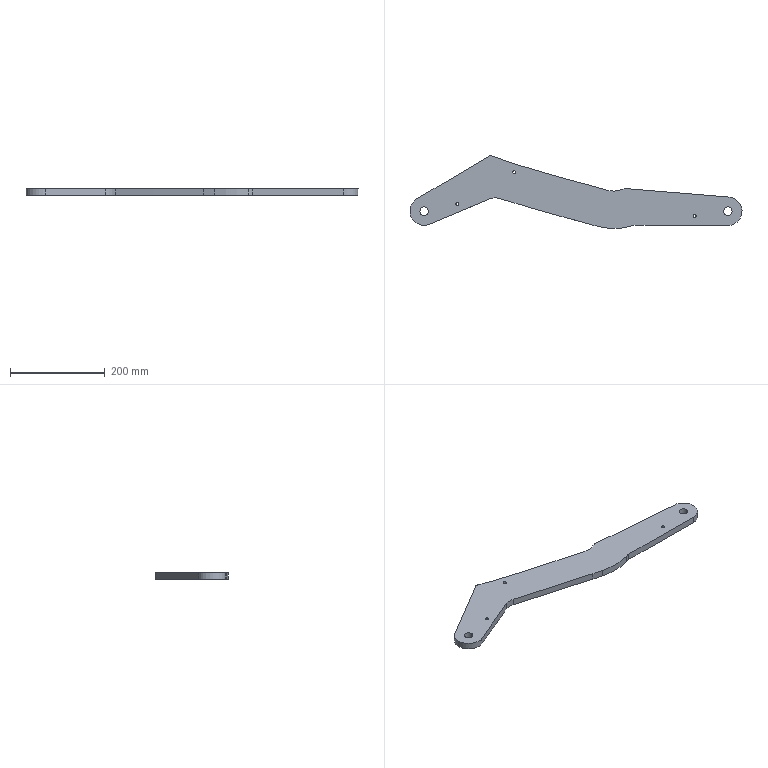Part | 1 solid | 30 faces | box 700 x 153.975 x 14 mm | volume 721262 mm3 | cylinder 14 | spline 10 | plane 6 | commonest cylinder face diameters 6.35 x6 18 x4 60 x4